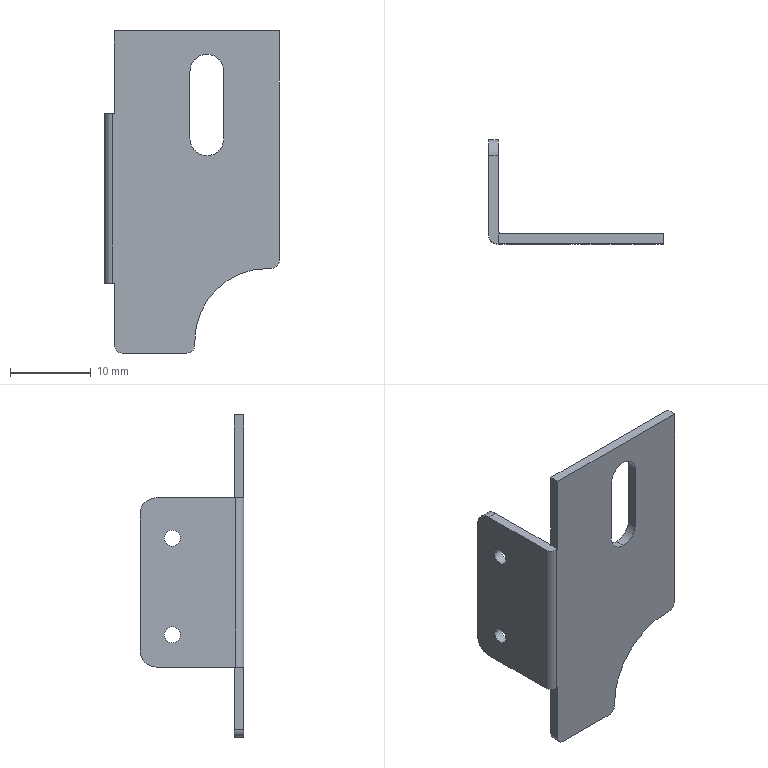Part | STEP file | ASND-0110-SDS_9 | 1 solid | 31 faces | box 21.7 x 12.9 x 40 mm | volume 1125 mm3 | plane 16 | cylinder 15 | commonest cylinder face diameters 2 x8 4.2 x3 4 x2 1 x1 18 x1